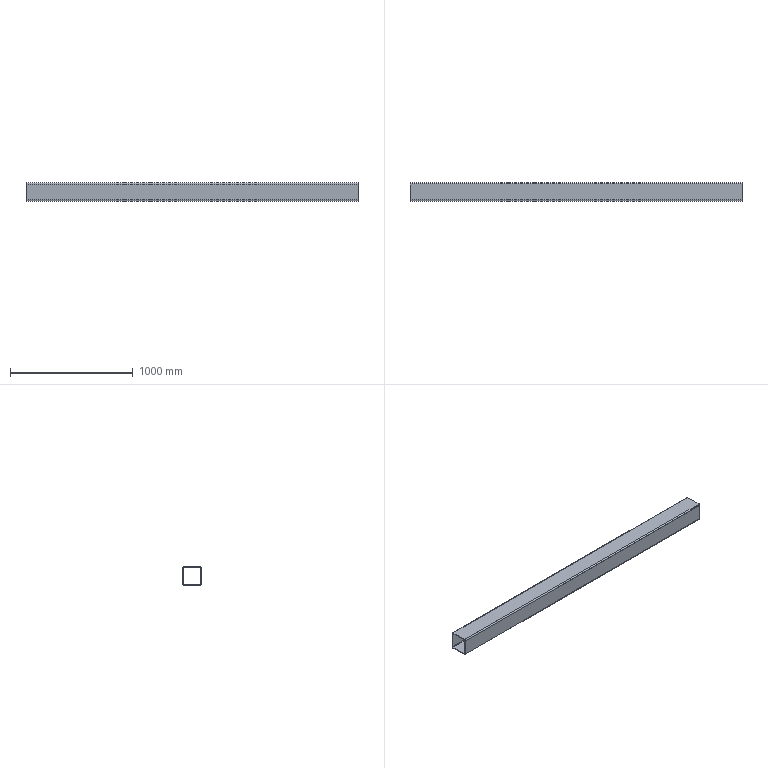Part | SolidWorks | features WeldMemberFeat 1, WeldmentFeature 1 | 1 solid | 18 faces | box 2700 x 150 x 150 mm | volume 7656173 mm3 | plane 10 | cylinder 8 | commonest cylinder face diameters 10 x4 20 x4
STEP:
#1=CARTESIAN_POINT('',(-1350.,75.,65.));
#2=VERTEX_POINT('',#1);
#3=CARTESIAN_POINT('',(-1350.,65.,75.));
#4=VERTEX_POINT('',#3);
#5=CARTESIAN_POINT('',(-1350.,65.,65.));
#6=DIRECTION('',(1.,0.,0.));
#7=DIRECTION('',(0.,1.,0.));
#8=AXIS2_PLACEMENT_3D('',#5,#6,#7);
#9=CIRCLE('',#8,10.);
#10=EDGE_CURVE('',#2,#4,#9,.T.);
#11=ORIENTED_EDGE('',*,*,#10,.T.);
#12=CARTESIAN_POINT('',(1350.,65.,75.));
#13=VERTEX_POINT('',#12);
#14=CARTESIAN_POINT('',(1350.,65.,75.));
#15=DIRECTION('',(-1.,0.,0.));
#16=VECTOR('',#15,1000.);
#17=LINE('',#14,#16);
#18=EDGE_CURVE('',#13,#4,#17,.T.);
#19=ORIENTED_EDGE('',*,*,#18,.F.);
#20=CARTESIAN_POINT('',(1350.,75.,65.));
#21=VERTEX_POINT('',#20);
#22=CARTESIAN_POINT('',(1350.,65.,65.));
#23=DIRECTION('',(1.,0.,0.));
#24=DIRECTION('',(0.,1.,0.));
#25=AXIS2_PLACEMENT_3D('',#22,#23,#24);
#26=CIRCLE('',#25,10.);
#27=EDGE_CURVE('',#21,#13,#26,.T.);
#28=ORIENTED_EDGE('',*,*,#27,.F.);
#29=CARTESIAN_POINT('',(1350.,75.,65.));
#30=DIRECTION('',(-1.,0.,0.));
#31=VECTOR('',#30,1000.);
#32=LINE('',#29,#31);
#33=EDGE_CURVE('',#21,#2,#32,.T.);
#34=ORIENTED_EDGE('',*,*,#33,.T.);
#35=EDGE_LOOP('',(#11,#19,#28,#34));
#36=FACE_OUTER_BOUND('',#35,.T.);
#37=CARTESIAN_POINT('',(1350.,65.,65.));
#38=DIRECTION('',(-1.,0.,0.));
#39=DIRECTION('',(0.,-1.,0.));
#40=AXIS2_PLACEMENT_3D('',#37,#38,#39);
#41=CYLINDRICAL_SURFACE('',#40,10.);
#42=ADVANCED_FACE('',(#36),#41,.T.);
#43=CARTESIAN_POINT('',(-1350.,-65.,75.));
#44=VERTEX_POINT('',#43);
#45=CARTESIAN_POINT('',(-1350.,65.,75.));
#46=DIRECTION('',(0.,-1.,0.));
#47=VECTOR('',#46,1000.);
#48=LINE('',#45,#47);
#49=EDGE_CURVE('',#4,#44,#48,.T.);
#50=ORIENTED_EDGE('',*,*,#49,.T.);
#51=CARTESIAN_POINT('',(1350.,-65.,75.));
#52=VERTEX_POINT('',#51);
#53=CARTESIAN_POINT('',(1350.,-65.,75.));
#54=DIRECTION('',(-1.,0.,0.));
#55=VECTOR('',#54,1000.);
#56=LINE('',#53,#55);
#57=EDGE_CURVE('',#52,#44,#56,.T.);
#58=ORIENTED_EDGE('',*,*,#57,.F.);
#59=CARTESIAN_POINT('',(1350.,65.,75.));
#60=DIRECTION('',(0.,-1.,0.));
#61=VECTOR('',#60,1000.);
#62=LINE('',#59,#61);
#63=EDGE_CURVE('',#13,#52,#62,.T.);
#64=ORIENTED_EDGE('',*,*,#63,.F.);
#65=ORIENTED_EDGE('',*,*,#18,.T.);
#66=EDGE_LOOP('',(#50,#58,#64,#65));
#67=FACE_OUTER_BOUND('',#66,.T.);
#68=CARTESIAN_POINT('',(1350.,65.,75.));
#69=DIRECTION('',(0.,0.,-1.));
#70=DIRECTION('',(-1.,0.,0.));
#71=AXIS2_PLACEMENT_3D('',#68,#69,#70);
#72=PLANE('',#71);
#73=ADVANCED_FACE('',(#67),#72,.F.);
#74=CARTESIAN_POINT('',(-1350.,-75.,65.));
#75=VERTEX_POINT('',#74);
#76=CARTESIAN_POINT('',(-1350.,-65.,65.));
#77=DIRECTION('',(1.,0.,0.));
#78=DIRECTION('',(0.,1.,0.));
#79=AXIS2_PLACEMENT_3D('',#76,#77,#78);
#80=CIRCLE('',#79,10.);
#81=EDGE_CURVE('',#44,#75,#80,.T.);
#82=ORIENTED_EDGE('',*,*,#81,.T.);
#83=CARTESIAN_POINT('',(1350.,-75.,65.));
#84=VERTEX_POINT('',#83);
#85=CARTESIAN_POINT('',(1350.,-75.,65.));
#86=DIRECTION('',(-1.,0.,0.));
#87=VECTOR('',#86,1000.);
#88=LINE('',#85,#87);
#89=EDGE_CURVE('',#84,#75,#88,.T.);
#90=ORIENTED_EDGE('',*,*,#89,.F.);
#91=CARTESIAN_POINT('',(1350.,-65.,65.));
#92=DIRECTION('',(1.,0.,0.));
#93=DIRECTION('',(0.,1.,0.));
#94=AXIS2_PLACEMENT_3D('',#91,#92,#93);
#95=CIRCLE('',#94,10.);
#96=EDGE_CURVE('',#52,#84,#95,.T.);
#97=ORIENTED_EDGE('',*,*,#96,.F.);
#98=ORIENTED_EDGE('',*,*,#57,.T.);
#99=EDGE_LOOP('',(#82,#90,#97,#98));
#100=FACE_OUTER_BOUND('',#99,.T.);
#101=CARTESIAN_POINT('',(1350.,-65.,65.));
#102=DIRECTION('',(-1.,0.,0.));
#103=DIRECTION('',(0.,-1.,0.));
#104=AXIS2_PLACEMENT_3D('',#101,#102,#103);
#105=CYLINDRICAL_SURFACE('',#104,10.);
#106=ADVANCED_FACE('',(#100),#105,.T.);
#107=CARTESIAN_POINT('',(-1350.,-75.,-65.));
#108=VERTEX_POINT('',#107);
#109=CARTESIAN_POINT('',(-1350.,-75.,-65.));
#110=DIRECTION('',(0.,0.,-1.));
#111=VECTOR('',#110,1000.);
#112=LINE('',#109,#111);
#113=EDGE_CURVE('',#75,#108,#112,.T.);
#114=ORIENTED_EDGE('',*,*,#113,.T.);
#115=CARTESIAN_POINT('',(1350.,-75.,-65.));
#116=VERTEX_POINT('',#115);
#117=CARTESIAN_POINT('',(1350.,-75.,-65.));
#118=DIRECTION('',(-1.,0.,0.));
#119=VECTOR('',#118,1000.);
#120=LINE('',#117,#119);
#121=EDGE_CURVE('',#116,#108,#120,.T.);
#122=ORIENTED_EDGE('',*,*,#121,.F.);
#123=CARTESIAN_POINT('',(1350.,-75.,-65.));
#124=DIRECTION('',(0.,0.,-1.));
#125=VECTOR('',#124,1000.);
#126=LINE('',#123,#125);
#127=EDGE_CURVE('',#84,#116,#126,.T.);
#128=ORIENTED_EDGE('',*,*,#127,.F.);
#129=ORIENTED_EDGE('',*,*,#89,.T.);
#130=EDGE_LOOP('',(#114,#122,#128,#129));
#131=FACE_OUTER_BOUND('',#130,.T.);
#132=CARTESIAN_POINT('',(1350.,-75.,-65.));
#133=DIRECTION('',(0.,1.,0.));
#134=DIRECTION('',(-1.,0.,0.));
#135=AXIS2_PLACEMENT_3D('',#132,#133,#134);
#136=PLANE('',#135);
#137=ADVANCED_FACE('',(#131),#136,.F.);
#138=CARTESIAN_POINT('',(-1350.,-65.,-75.));
#139=VERTEX_POINT('',#138);
#140=CARTESIAN_POINT('',(-1350.,-65.,-65.));
#141=DIRECTION('',(1.,0.,0.));
#142=DIRECTION('',(0.,1.,0.));
#143=AXIS2_PLACEMENT_3D('',#140,#141,#142);
#144=CIRCLE('',#143,10.);
#145=EDGE_CURVE('',#108,#139,#144,.T.);
#146=ORIENTED_EDGE('',*,*,#145,.T.);
#147=CARTESIAN_POINT('',(1350.,-65.,-75.));
#148=VERTEX_POINT('',#147);
#149=CARTESIAN_POINT('',(1350.,-65.,-75.));
#150=DIRECTION('',(-1.,0.,0.));
#151=VECTOR('',#150,1000.);
#152=LINE('',#149,#151);
#153=EDGE_CURVE('',#148,#139,#152,.T.);
#154=ORIENTED_EDGE('',*,*,#153,.F.);
#155=CARTESIAN_POINT('',(1350.,-65.,-65.));
#156=DIRECTION('',(1.,0.,0.));
#157=DIRECTION('',(0.,1.,0.));
#158=AXIS2_PLACEMENT_3D('',#155,#156,#157);
#159=CIRCLE('',#158,10.);
#160=EDGE_CURVE('',#116,#148,#159,.T.);
#161=ORIENTED_EDGE('',*,*,#160,.F.);
#162=ORIENTED_EDGE('',*,*,#121,.T.);
#163=EDGE_LOOP('',(#146,#154,#161,#162));
#164=FACE_OUTER_BOUND('',#163,.T.);
#165=CARTESIAN_POINT('',(1350.,-65.,-65.));
#166=DIRECTION('',(-1.,0.,0.));
#167=DIRECTION('',(0.,-1.,0.));
#168=AXIS2_PLACEMENT_3D('',#165,#166,#167);
#169=CYLINDRICAL_SURFACE('',#168,10.);
#170=ADVANCED_FACE('',(#164),#169,.T.);
#171=CARTESIAN_POINT('',(-1350.,65.,-75.));
#172=VERTEX_POINT('',#171);
#173=CARTESIAN_POINT('',(-1350.,-65.,-75.));
#174=DIRECTION('',(0.,1.,0.));
#175=VECTOR('',#174,1000.);
#176=LINE('',#173,#175);
#177=EDGE_CURVE('',#139,#172,#176,.T.);
#178=ORIENTED_EDGE('',*,*,#177,.T.);
#179=CARTESIAN_POINT('',(1350.,65.,-75.));
#180=VERTEX_POINT('',#179);
#181=CARTESIAN_POINT('',(1350.,65.,-75.));
#182=DIRECTION('',(-1.,0.,0.));
#183=VECTOR('',#182,1000.);
#184=LINE('',#181,#183);
#185=EDGE_CURVE('',#180,#172,#184,.T.);
#186=ORIENTED_EDGE('',*,*,#185,.F.);
#187=CARTESIAN_POINT('',(1350.,-65.,-75.));
#188=DIRECTION('',(0.,1.,0.));
#189=VECTOR('',#188,1000.);
#190=LINE('',#187,#189);
#191=EDGE_CURVE('',#148,#180,#190,.T.);
#192=ORIENTED_EDGE('',*,*,#191,.F.);
#193=ORIENTED_EDGE('',*,*,#153,.T.);
#194=EDGE_LOOP('',(#178,#186,#192,#193));
#195=FACE_OUTER_BOUND('',#194,.T.);
#196=CARTESIAN_POINT('',(1350.,-65.,-75.));
#197=DIRECTION('',(0.,0.,1.));
#198=DIRECTION('',(1.,0.,0.));
#199=AXIS2_PLACEMENT_3D('',#196,#197,#198);
#200=PLANE('',#199);
#201=ADVANCED_FACE('',(#195),#200,.F.);
#202=CARTESIAN_POINT('',(-1350.,75.,-65.));
#203=VERTEX_POINT('',#202);
#204=CARTESIAN_POINT('',(-1350.,65.,-65.));
#205=DIRECTION('',(1.,0.,0.));
#206=DIRECTION('',(0.,1.,0.));
#207=AXIS2_PLACEMENT_3D('',#204,#205,#206);
#208=CIRCLE('',#207,10.);
#209=EDGE_CURVE('',#172,#203,#208,.T.);
#210=ORIENTED_EDGE('',*,*,#209,.T.);
#211=CARTESIAN_POINT('',(1350.,75.,-65.));
#212=VERTEX_POINT('',#211);
#213=CARTESIAN_POINT('',(1350.,75.,-65.));
#214=DIRECTION('',(-1.,0.,0.));
#215=VECTOR('',#214,1000.);
#216=LINE('',#213,#215);
#217=EDGE_CURVE('',#212,#203,#216,.T.);
#218=ORIENTED_EDGE('',*,*,#217,.F.);
#219=CARTESIAN_POINT('',(1350.,65.,-65.));
#220=DIRECTION('',(1.,0.,0.));
#221=DIRECTION('',(0.,1.,0.));
#222=AXIS2_PLACEMENT_3D('',#219,#220,#221);
#223=CIRCLE('',#222,10.);
#224=EDGE_CURVE('',#180,#212,#223,.T.);
#225=ORIENTED_EDGE('',*,*,#224,.F.);
#226=ORIENTED_EDGE('',*,*,#185,.T.);
#227=EDGE_LOOP('',(#210,#218,#225,#226));
#228=FACE_OUTER_BOUND('',#227,.T.);
#229=CARTESIAN_POINT('',(1350.,65.,-65.));
#230=DIRECTION('',(-1.,0.,0.));
#231=DIRECTION('',(0.,-1.,0.));
#232=AXIS2_PLACEMENT_3D('',#229,#230,#231);
#233=CYLINDRICAL_SURFACE('',#232,10.);
#234=ADVANCED_FACE('',(#228),#233,.T.);
#235=CARTESIAN_POINT('',(-1350.,-65.,70.));
#236=VERTEX_POINT('',#235);
#237=CARTESIAN_POINT('',(-1350.,-70.,65.));
#238=VERTEX_POINT('',#237);
#239=CARTESIAN_POINT('',(-1350.,-65.,65.));
#240=DIRECTION('',(1.,0.,0.));
#241=DIRECTION('',(0.,1.,0.));
#242=AXIS2_PLACEMENT_3D('',#239,#240,#241);
#243=CIRCLE('',#242,5.);
#244=EDGE_CURVE('',#236,#238,#243,.T.);
#245=ORIENTED_EDGE('',*,*,#244,.F.);
#246=CARTESIAN_POINT('',(1350.,-65.,70.));
#247=VERTEX_POINT('',#246);
#248=CARTESIAN_POINT('',(1350.,-65.,70.));
#249=DIRECTION('',(-1.,0.,0.));
#250=VECTOR('',#249,1000.);
#251=LINE('',#248,#250);
#252=EDGE_CURVE('',#247,#236,#251,.T.);
#253=ORIENTED_EDGE('',*,*,#252,.F.);
#254=CARTESIAN_POINT('',(1350.,-70.,65.));
#255=VERTEX_POINT('',#254);
#256=CARTESIAN_POINT('',(1350.,-65.,65.));
#257=DIRECTION('',(1.,0.,0.));
#258=DIRECTION('',(0.,1.,0.));
#259=AXIS2_PLACEMENT_3D('',#256,#257,#258);
#260=CIRCLE('',#259,5.);
#261=EDGE_CURVE('',#247,#255,#260,.T.);
#262=ORIENTED_EDGE('',*,*,#261,.T.);
#263=CARTESIAN_POINT('',(1350.,-70.,65.));
#264=DIRECTION('',(-1.,0.,0.));
#265=VECTOR('',#264,1000.);
#266=LINE('',#263,#265);
#267=EDGE_CURVE('',#255,#238,#266,.T.);
#268=ORIENTED_EDGE('',*,*,#267,.T.);
#269=EDGE_LOOP('',(#245,#253,#262,#268));
#270=FACE_OUTER_BOUND('',#269,.T.);
#271=CARTESIAN_POINT('',(1350.,-65.,65.));
#272=DIRECTION('',(-1.,0.,0.));
#273=DIRECTION('',(0.,-1.,0.));
#274=AXIS2_PLACEMENT_3D('',#271,#272,#273);
#275=CYLINDRICAL_SURFACE('',#274,5.);
#276=ADVANCED_FACE('',(#270),#275,.F.);
#277=CARTESIAN_POINT('',(-1350.,65.,70.));
#278=VERTEX_POINT('',#277);
#279=CARTESIAN_POINT('',(-1350.,65.,70.));
#280=DIRECTION('',(0.,-1.,0.));
#281=VECTOR('',#280,1000.);
#282=LINE('',#279,#281);
#283=EDGE_CURVE('',#278,#236,#282,.T.);
#284=ORIENTED_EDGE('',*,*,#283,.F.);
#285=CARTESIAN_POINT('',(1350.,65.,70.));
#286=VERTEX_POINT('',#285);
#287=CARTESIAN_POINT('',(1350.,65.,70.));
#288=DIRECTION('',(-1.,0.,0.));
#289=VECTOR('',#288,1000.);
#290=LINE('',#287,#289);
#291=EDGE_CURVE('',#286,#278,#290,.T.);
#292=ORIENTED_EDGE('',*,*,#291,.F.);
#293=CARTESIAN_POINT('',(1350.,65.,70.));
#294=DIRECTION('',(0.,-1.,0.));
#295=VECTOR('',#294,1000.);
#296=LINE('',#293,#295);
#297=EDGE_CURVE('',#286,#247,#296,.T.);
#298=ORIENTED_EDGE('',*,*,#297,.T.);
#299=ORIENTED_EDGE('',*,*,#252,.T.);
#300=EDGE_LOOP('',(#284,#292,#298,#299));
#301=FACE_OUTER_BOUND('',#300,.T.);
#302=CARTESIAN_POINT('',(1350.,65.,70.));
#303=DIRECTION('',(0.,0.,-1.));
#304=DIRECTION('',(-1.,0.,0.));
#305=AXIS2_PLACEMENT_3D('',#302,#303,#304);
#306=PLANE('',#305);
#307=ADVANCED_FACE('',(#301),#306,.T.);
#308=CARTESIAN_POINT('',(-1350.,70.,65.));
#309=VERTEX_POINT('',#308);
#310=CARTESIAN_POINT('',(-1350.,65.,65.));
#311=DIRECTION('',(1.,0.,0.));
#312=DIRECTION('',(0.,1.,0.));
#313=AXIS2_PLACEMENT_3D('',#310,#311,#312);
#314=CIRCLE('',#313,5.);
#315=EDGE_CURVE('',#309,#278,#314,.T.);
#316=ORIENTED_EDGE('',*,*,#315,.F.);
#317=CARTESIAN_POINT('',(1350.,70.,65.));
#318=VERTEX_POINT('',#317);
#319=CARTESIAN_POINT('',(1350.,70.,65.));
#320=DIRECTION('',(-1.,0.,0.));
#321=VECTOR('',#320,1000.);
#322=LINE('',#319,#321);
#323=EDGE_CURVE('',#318,#309,#322,.T.);
#324=ORIENTED_EDGE('',*,*,#323,.F.);
#325=CARTESIAN_POINT('',(1350.,65.,65.));
#326=DIRECTION('',(1.,0.,0.));
#327=DIRECTION('',(0.,1.,0.));
#328=AXIS2_PLACEMENT_3D('',#325,#326,#327);
#329=CIRCLE('',#328,5.);
#330=EDGE_CURVE('',#318,#286,#329,.T.);
#331=ORIENTED_EDGE('',*,*,#330,.T.);
#332=ORIENTED_EDGE('',*,*,#291,.T.);
#333=EDGE_LOOP('',(#316,#324,#331,#332));
#334=FACE_OUTER_BOUND('',#333,.T.);
#335=CARTESIAN_POINT('',(1350.,65.,65.));
#336=DIRECTION('',(-1.,0.,0.));
#337=DIRECTION('',(0.,-1.,0.));
#338=AXIS2_PLACEMENT_3D('',#335,#336,#337);
#339=CYLINDRICAL_SURFACE('',#338,5.);
#340=ADVANCED_FACE('',(#334),#339,.F.);
#341=CARTESIAN_POINT('',(-1350.,70.,-65.));
#342=VERTEX_POINT('',#341);
#343=CARTESIAN_POINT('',(-1350.,70.,65.));
#344=DIRECTION('',(0.,0.,1.));
#345=VECTOR('',#344,1000.);
#346=LINE('',#343,#345);
#347=EDGE_CURVE('',#342,#309,#346,.T.);
#348=ORIENTED_EDGE('',*,*,#347,.F.);
#349=CARTESIAN_POINT('',(1350.,70.,-65.));
#350=VERTEX_POINT('',#349);
#351=CARTESIAN_POINT('',(1350.,70.,-65.));
#352=DIRECTION('',(-1.,0.,0.));
#353=VECTOR('',#352,1000.);
#354=LINE('',#351,#353);
#355=EDGE_CURVE('',#350,#342,#354,.T.);
#356=ORIENTED_EDGE('',*,*,#355,.F.);
#357=CARTESIAN_POINT('',(1350.,70.,65.));
#358=DIRECTION('',(0.,0.,1.));
#359=VECTOR('',#358,1000.);
#360=LINE('',#357,#359);
#361=EDGE_CURVE('',#350,#318,#360,.T.);
#362=ORIENTED_EDGE('',*,*,#361,.T.);
#363=ORIENTED_EDGE('',*,*,#323,.T.);
#364=EDGE_LOOP('',(#348,#356,#362,#363));
#365=FACE_OUTER_BOUND('',#364,.T.);
#366=CARTESIAN_POINT('',(1350.,70.,65.));
#367=DIRECTION('',(0.,-1.,0.));
#368=DIRECTION('',(1.,0.,0.));
#369=AXIS2_PLACEMENT_3D('',#366,#367,#368);
#370=PLANE('',#369);
#371=ADVANCED_FACE('',(#365),#370,.T.);
#372=CARTESIAN_POINT('',(-1350.,65.,-70.));
#373=VERTEX_POINT('',#372);
#374=CARTESIAN_POINT('',(-1350.,65.,-65.));
#375=DIRECTION('',(1.,0.,0.));
#376=DIRECTION('',(0.,1.,0.));
#377=AXIS2_PLACEMENT_3D('',#374,#375,#376);
#378=CIRCLE('',#377,5.);
#379=EDGE_CURVE('',#373,#342,#378,.T.);
#380=ORIENTED_EDGE('',*,*,#379,.F.);
#381=CARTESIAN_POINT('',(1350.,65.,-70.));
#382=VERTEX_POINT('',#381);
#383=CARTESIAN_POINT('',(1350.,65.,-70.));
#384=DIRECTION('',(-1.,0.,0.));
#385=VECTOR('',#384,1000.);
#386=LINE('',#383,#385);
#387=EDGE_CURVE('',#382,#373,#386,.T.);
#388=ORIENTED_EDGE('',*,*,#387,.F.);
#389=CARTESIAN_POINT('',(1350.,65.,-65.));
#390=DIRECTION('',(1.,0.,0.));
#391=DIRECTION('',(0.,1.,0.));
#392=AXIS2_PLACEMENT_3D('',#389,#390,#391);
#393=CIRCLE('',#392,5.);
#394=EDGE_CURVE('',#382,#350,#393,.T.);
#395=ORIENTED_EDGE('',*,*,#394,.T.);
#396=ORIENTED_EDGE('',*,*,#355,.T.);
#397=EDGE_LOOP('',(#380,#388,#395,#396));
#398=FACE_OUTER_BOUND('',#397,.T.);
#399=CARTESIAN_POINT('',(1350.,65.,-65.));
#400=DIRECTION('',(-1.,0.,0.));
#401=DIRECTION('',(0.,-1.,0.));
#402=AXIS2_PLACEMENT_3D('',#399,#400,#401);
#403=CYLINDRICAL_SURFACE('',#402,5.);
#404=ADVANCED_FACE('',(#398),#403,.F.);
#405=CARTESIAN_POINT('',(-1350.,-65.,-70.));
#406=VERTEX_POINT('',#405);
#407=CARTESIAN_POINT('',(-1350.,-65.,-70.));
#408=DIRECTION('',(0.,1.,0.));
#409=VECTOR('',#408,1000.);
#410=LINE('',#407,#409);
#411=EDGE_CURVE('',#406,#373,#410,.T.);
#412=ORIENTED_EDGE('',*,*,#411,.F.);
#413=CARTESIAN_POINT('',(1350.,-65.,-70.));
#414=VERTEX_POINT('',#413);
#415=CARTESIAN_POINT('',(1350.,-65.,-70.));
#416=DIRECTION('',(-1.,0.,0.));
#417=VECTOR('',#416,1000.);
#418=LINE('',#415,#417);
#419=EDGE_CURVE('',#414,#406,#418,.T.);
#420=ORIENTED_EDGE('',*,*,#419,.F.);
#421=CARTESIAN_POINT('',(1350.,-65.,-70.));
#422=DIRECTION('',(0.,1.,0.));
#423=VECTOR('',#422,1000.);
#424=LINE('',#421,#423);
#425=EDGE_CURVE('',#414,#382,#424,.T.);
#426=ORIENTED_EDGE('',*,*,#425,.T.);
#427=ORIENTED_EDGE('',*,*,#387,.T.);
#428=EDGE_LOOP('',(#412,#420,#426,#427));
#429=FACE_OUTER_BOUND('',#428,.T.);
#430=CARTESIAN_POINT('',(1350.,-65.,-70.));
#431=DIRECTION('',(0.,0.,1.));
#432=DIRECTION('',(1.,0.,0.));
#433=AXIS2_PLACEMENT_3D('',#430,#431,#432);
#434=PLANE('',#433);
#435=ADVANCED_FACE('',(#429),#434,.T.);
#436=CARTESIAN_POINT('',(-1350.,-70.,-65.));
#437=VERTEX_POINT('',#436);
#438=CARTESIAN_POINT('',(-1350.,-65.,-65.));
#439=DIRECTION('',(1.,0.,0.));
#440=DIRECTION('',(0.,1.,0.));
#441=AXIS2_PLACEMENT_3D('',#438,#439,#440);
#442=CIRCLE('',#441,5.);
#443=EDGE_CURVE('',#437,#406,#442,.T.);
#444=ORIENTED_EDGE('',*,*,#443,.F.);
#445=CARTESIAN_POINT('',(1350.,-70.,-65.));
#446=VERTEX_POINT('',#445);
#447=CARTESIAN_POINT('',(1350.,-70.,-65.));
#448=DIRECTION('',(-1.,0.,0.));
#449=VECTOR('',#448,1000.);
#450=LINE('',#447,#449);
#451=EDGE_CURVE('',#446,#437,#450,.T.);
#452=ORIENTED_EDGE('',*,*,#451,.F.);
#453=CARTESIAN_POINT('',(1350.,-65.,-65.));
#454=DIRECTION('',(1.,0.,0.));
#455=DIRECTION('',(0.,1.,0.));
#456=AXIS2_PLACEMENT_3D('',#453,#454,#455);
#457=CIRCLE('',#456,5.);
#458=EDGE_CURVE('',#446,#414,#457,.T.);
#459=ORIENTED_EDGE('',*,*,#458,.T.);
#460=ORIENTED_EDGE('',*,*,#419,.T.);
#461=EDGE_LOOP('',(#444,#452,#459,#460));
#462=FACE_OUTER_BOUND('',#461,.T.);
#463=CARTESIAN_POINT('',(1350.,-65.,-65.));
#464=DIRECTION('',(-1.,0.,0.));
#465=DIRECTION('',(0.,-1.,0.));
#466=AXIS2_PLACEMENT_3D('',#463,#464,#465);
#467=CYLINDRICAL_SURFACE('',#466,5.);
#468=ADVANCED_FACE('',(#462),#467,.F.);
#469=CARTESIAN_POINT('',(-1350.,-70.,-65.));
#470=DIRECTION('',(0.,0.,-1.));
#471=VECTOR('',#470,1000.);
#472=LINE('',#469,#471);
#473=EDGE_CURVE('',#238,#437,#472,.T.);
#474=ORIENTED_EDGE('',*,*,#473,.F.);
#475=ORIENTED_EDGE('',*,*,#267,.F.);
#476=CARTESIAN_POINT('',(1350.,-70.,-65.));
#477=DIRECTION('',(0.,0.,-1.));
#478=VECTOR('',#477,1000.);
#479=LINE('',#476,#478);
#480=EDGE_CURVE('',#255,#446,#479,.T.);
#481=ORIENTED_EDGE('',*,*,#480,.T.);
#482=ORIENTED_EDGE('',*,*,#451,.T.);
#483=EDGE_LOOP('',(#474,#475,#481,#482));
#484=FACE_OUTER_BOUND('',#483,.T.);
#485=CARTESIAN_POINT('',(1350.,-70.,-65.));
#486=DIRECTION('',(0.,1.,0.));
#487=DIRECTION('',(-1.,0.,0.));
#488=AXIS2_PLACEMENT_3D('',#485,#486,#487);
#489=PLANE('',#488);
#490=ADVANCED_FACE('',(#484),#489,.T.);
#491=CARTESIAN_POINT('',(-1350.,75.,65.));
#492=DIRECTION('',(0.,0.,1.));
#493=VECTOR('',#492,1000.);
#494=LINE('',#491,#493);
#495=EDGE_CURVE('',#203,#2,#494,.T.);
#496=ORIENTED_EDGE('',*,*,#495,.T.);
#497=ORIENTED_EDGE('',*,*,#33,.F.);
#498=CARTESIAN_POINT('',(1350.,75.,65.));
#499=DIRECTION('',(0.,0.,1.));
#500=VECTOR('',#499,1000.);
#501=LINE('',#498,#500);
#502=EDGE_CURVE('',#212,#21,#501,.T.);
#503=ORIENTED_EDGE('',*,*,#502,.F.);
#504=ORIENTED_EDGE('',*,*,#217,.T.);
#505=EDGE_LOOP('',(#496,#497,#503,#504));
#506=FACE_OUTER_BOUND('',#505,.T.);
#507=CARTESIAN_POINT('',(1350.,75.,65.));
#508=DIRECTION('',(0.,-1.,0.));
#509=DIRECTION('',(1.,0.,0.));
#510=AXIS2_PLACEMENT_3D('',#507,#508,#509);
#511=PLANE('',#510);
#512=ADVANCED_FACE('',(#506),#511,.F.);
#513=ORIENTED_EDGE('',*,*,#261,.F.);
#514=ORIENTED_EDGE('',*,*,#297,.F.);
#515=ORIENTED_EDGE('',*,*,#330,.F.);
#516=ORIENTED_EDGE('',*,*,#361,.F.);
#517=ORIENTED_EDGE('',*,*,#394,.F.);
#518=ORIENTED_EDGE('',*,*,#425,.F.);
#519=ORIENTED_EDGE('',*,*,#458,.F.);
#520=ORIENTED_EDGE('',*,*,#480,.F.);
#521=EDGE_LOOP('',(#513,#514,#515,#516,#517,#518,#519,#520));
#522=FACE_BOUND('',#521,.T.);
#523=ORIENTED_EDGE('',*,*,#27,.T.);
#524=ORIENTED_EDGE('',*,*,#63,.T.);
#525=ORIENTED_EDGE('',*,*,#96,.T.);
#526=ORIENTED_EDGE('',*,*,#127,.T.);
#527=ORIENTED_EDGE('',*,*,#160,.T.);
#528=ORIENTED_EDGE('',*,*,#191,.T.);
#529=ORIENTED_EDGE('',*,*,#224,.T.);
#530=ORIENTED_EDGE('',*,*,#502,.T.);
#531=EDGE_LOOP('',(#523,#524,#525,#526,#527,#528,#529,#530));
#532=FACE_OUTER_BOUND('',#531,.T.);
#533=CARTESIAN_POINT('',(1350.,65.,65.));
#534=DIRECTION('',(1.,0.,0.));
#535=DIRECTION('',(0.,1.,0.));
#536=AXIS2_PLACEMENT_3D('',#533,#534,#535);
#537=PLANE('',#536);
#538=ADVANCED_FACE('',(#522,#532),#537,.T.);
#539=ORIENTED_EDGE('',*,*,#244,.T.);
#540=ORIENTED_EDGE('',*,*,#473,.T.);
#541=ORIENTED_EDGE('',*,*,#443,.T.);
#542=ORIENTED_EDGE('',*,*,#411,.T.);
#543=ORIENTED_EDGE('',*,*,#379,.T.);
#544=ORIENTED_EDGE('',*,*,#347,.T.);
#545=ORIENTED_EDGE('',*,*,#315,.T.);
#546=ORIENTED_EDGE('',*,*,#283,.T.);
#547=EDGE_LOOP('',(#539,#540,#541,#542,#543,#544,#545,#546));
#548=FACE_BOUND('',#547,.T.);
#549=ORIENTED_EDGE('',*,*,#10,.F.);
#550=ORIENTED_EDGE('',*,*,#495,.F.);
#551=ORIENTED_EDGE('',*,*,#209,.F.);
#552=ORIENTED_EDGE('',*,*,#177,.F.);
#553=ORIENTED_EDGE('',*,*,#145,.F.);
#554=ORIENTED_EDGE('',*,*,#113,.F.);
#555=ORIENTED_EDGE('',*,*,#81,.F.);
#556=ORIENTED_EDGE('',*,*,#49,.F.);
#557=EDGE_LOOP('',(#549,#550,#551,#552,#553,#554,#555,#556));
#558=FACE_OUTER_BOUND('',#557,.T.);
#559=CARTESIAN_POINT('',(-1350.,65.,65.));
#560=DIRECTION('',(1.,0.,0.));
#561=DIRECTION('',(0.,1.,0.));
#562=AXIS2_PLACEMENT_3D('',#559,#560,#561);
#563=PLANE('',#562);
#564=ADVANCED_FACE('',(#548,#558),#563,.F.);
#565=CLOSED_SHELL('',(#42,#73,#106,#137,#170,#201,#234,#276,#307,#340,#371,#404,#435,#468,#490,#512,#538,#564));
#566=MANIFOLD_SOLID_BREP('',#565);
#567=CARTESIAN_POINT('',(0.,0.,0.));
#568=DIRECTION('',(0.,0.,1.));
#569=DIRECTION('',(1.,0.,0.));
#570=AXIS2_PLACEMENT_3D('',#567,#568,#569);
#571=(LENGTH_UNIT()NAMED_UNIT(*)SI_UNIT(.MILLI.,.METRE.));
#572=UNCERTAINTY_MEASURE_WITH_UNIT(LENGTH_MEASURE(0.00001),#571,'','');
#573=(NAMED_UNIT(*)PLANE_ANGLE_UNIT()SI_UNIT($,.RADIAN.));
#574=(NAMED_UNIT(*)SI_UNIT($,.STERADIAN.)SOLID_ANGLE_UNIT());
#575=(GEOMETRIC_REPRESENTATION_CONTEXT(3)GLOBAL_UNCERTAINTY_ASSIGNED_CONTEXT((#572))GLOBAL_UNIT_ASSIGNED_CONTEXT((#571,#573,#574))REPRESENTATION_CONTEXT('',''));
#576=ADVANCED_BREP_SHAPE_REPRESENTATION('',(#566,#570),#575);